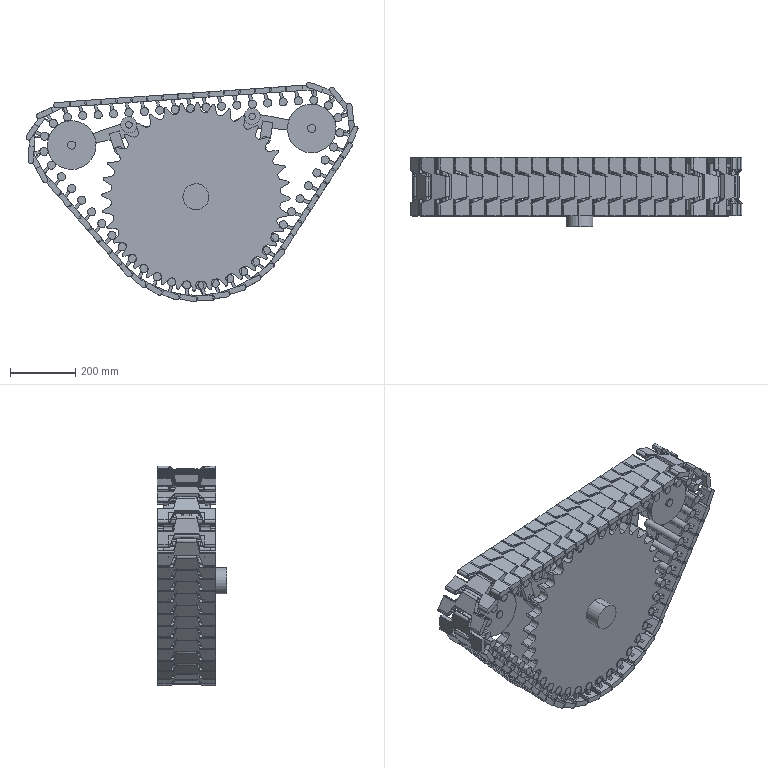Part | SolidWorks | features ReferencePattern 84, CompositeCurve 2, LocalChainPattern 1, LocalCirPattern 1, RefAxis 1 | 58 solids | 3399 faces | volume 31623376 mm3 | plane 1887 | cylinder 1500 | cone 8 | torus 4 | commonest cylinder face diameters 8 x600 25 x318 16 x300 4 x200 18 x16 20 x16